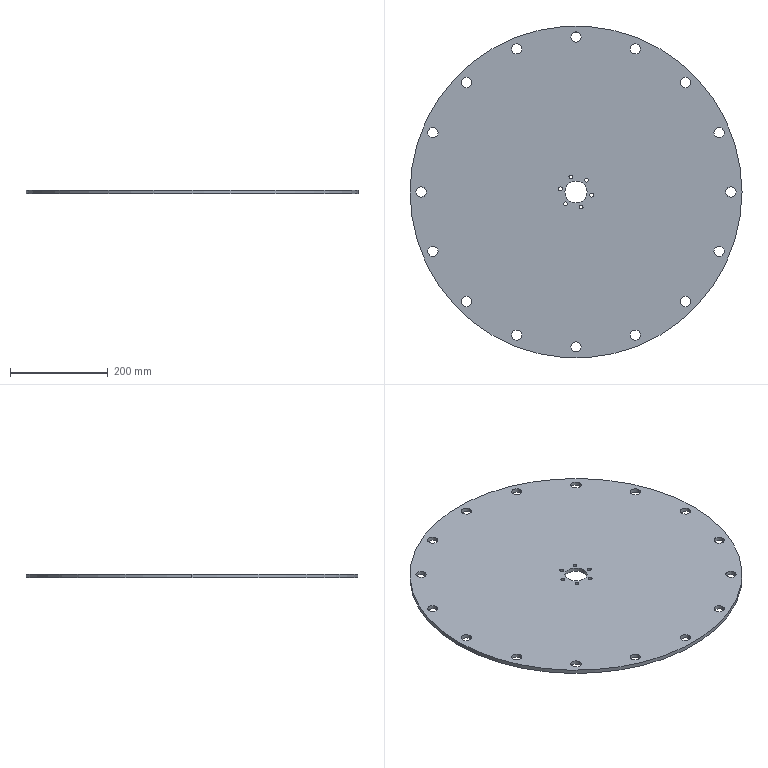Part | 1 solid | 50 faces | box 680 x 680 x 8 mm | volume 2845761 mm3 | cylinder 48 | plane 2 | commonest cylinder face diameters 21 x32 8 x12 45.2 x2 680 x2